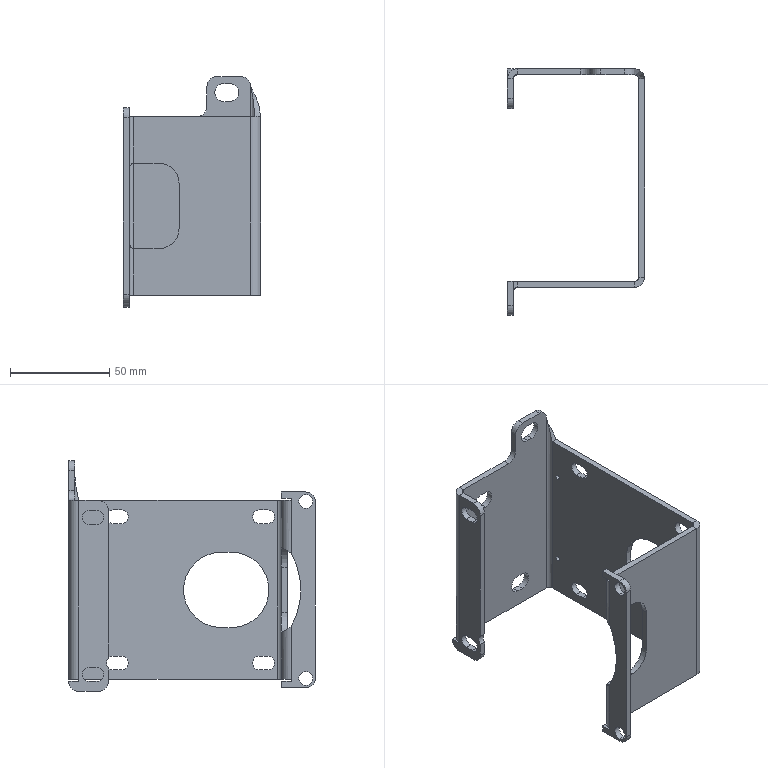Part | SolidWorks | features ICE 14, EdgeFlange 3, HoleWzd 2, FlatPattern 1, SM3dBend 1, SMBaseFlange 1, SheetMetal 1 | 1 solid | 122 faces | box 69 x 124 x 116 mm | volume 64085 mm3 | plane 62 | cylinder 53 | spline 7 | commonest cylinder face diameters 7 x17 10 x11 9 x6 4 x5 2.5 x4 1 x3